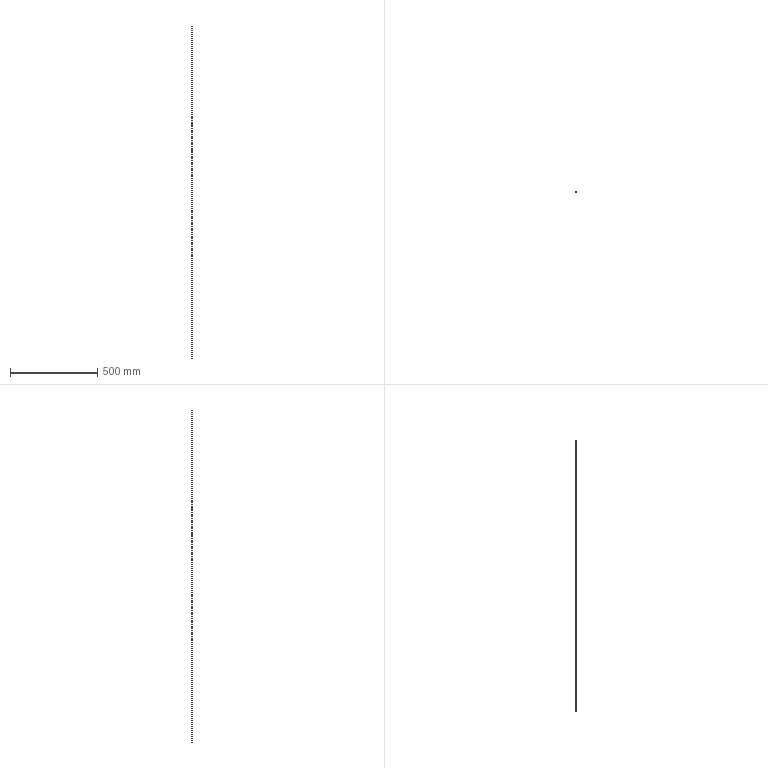Part | SolidWorks | features Extrusion 1 | 1 solid | 10 faces | box 3 x 3 x 1900 mm | volume 13027 mm3 | cylinder 8 | plane 2 | commonest cylinder face diameters 0.3 x6 3 x2
STEP:
#1=CARTESIAN_POINT('',(-0.9727,-0.475,1900.));
#2=VERTEX_POINT('',#1);
#3=CARTESIAN_POINT('',(-0.6727,-0.475,1900.));
#4=VERTEX_POINT('',#3);
#5=CARTESIAN_POINT('',(-0.8227,-0.475,1900.));
#6=DIRECTION('',(0.,0.,1.));
#7=DIRECTION('',(1.,0.,0.));
#8=AXIS2_PLACEMENT_3D('',#5,#6,#7);
#9=CIRCLE('',#8,0.15);
#10=EDGE_CURVE('',#2,#4,#9,.T.);
#11=ORIENTED_EDGE('',*,*,#10,.T.);
#12=CARTESIAN_POINT('',(-0.6727,-0.475,0.));
#13=VERTEX_POINT('',#12);
#14=CARTESIAN_POINT('',(-0.6727,-0.475,1900.));
#15=DIRECTION('',(0.,0.,-1.));
#16=VECTOR('',#15,1000.);
#17=LINE('',#14,#16);
#18=EDGE_CURVE('',#4,#13,#17,.T.);
#19=ORIENTED_EDGE('',*,*,#18,.T.);
#20=CARTESIAN_POINT('',(-0.9727,-0.475,0.));
#21=VERTEX_POINT('',#20);
#22=CARTESIAN_POINT('',(-0.8227,-0.475,0.));
#23=DIRECTION('',(0.,0.,1.));
#24=DIRECTION('',(1.,0.,0.));
#25=AXIS2_PLACEMENT_3D('',#22,#23,#24);
#26=CIRCLE('',#25,0.15);
#27=EDGE_CURVE('',#21,#13,#26,.T.);
#28=ORIENTED_EDGE('',*,*,#27,.F.);
#29=CARTESIAN_POINT('',(-0.9727,-0.475,1900.));
#30=DIRECTION('',(0.,0.,-1.));
#31=VECTOR('',#30,1000.);
#32=LINE('',#29,#31);
#33=EDGE_CURVE('',#2,#21,#32,.T.);
#34=ORIENTED_EDGE('',*,*,#33,.F.);
#35=EDGE_LOOP('',(#11,#19,#28,#34));
#36=FACE_OUTER_BOUND('',#35,.T.);
#37=CARTESIAN_POINT('',(-0.8227,-0.475,1900.));
#38=DIRECTION('',(0.,0.,-1.));
#39=DIRECTION('',(-1.,0.,0.));
#40=AXIS2_PLACEMENT_3D('',#37,#38,#39);
#41=CYLINDRICAL_SURFACE('',#40,0.15);
#42=ADVANCED_FACE('',(#36),#41,.F.);
#43=CARTESIAN_POINT('',(0.6727,-0.475,1900.));
#44=VERTEX_POINT('',#43);
#45=CARTESIAN_POINT('',(0.9727,-0.475,1900.));
#46=VERTEX_POINT('',#45);
#47=CARTESIAN_POINT('',(0.8227,-0.475,1900.));
#48=DIRECTION('',(0.,0.,1.));
#49=DIRECTION('',(1.,0.,0.));
#50=AXIS2_PLACEMENT_3D('',#47,#48,#49);
#51=CIRCLE('',#50,0.15);
#52=EDGE_CURVE('',#44,#46,#51,.T.);
#53=ORIENTED_EDGE('',*,*,#52,.T.);
#54=CARTESIAN_POINT('',(0.9727,-0.475,0.));
#55=VERTEX_POINT('',#54);
#56=CARTESIAN_POINT('',(0.9727,-0.475,1900.));
#57=DIRECTION('',(0.,0.,-1.));
#58=VECTOR('',#57,1000.);
#59=LINE('',#56,#58);
#60=EDGE_CURVE('',#46,#55,#59,.T.);
#61=ORIENTED_EDGE('',*,*,#60,.T.);
#62=CARTESIAN_POINT('',(0.6727,-0.475,0.));
#63=VERTEX_POINT('',#62);
#64=CARTESIAN_POINT('',(0.8227,-0.475,0.));
#65=DIRECTION('',(0.,0.,1.));
#66=DIRECTION('',(1.,0.,0.));
#67=AXIS2_PLACEMENT_3D('',#64,#65,#66);
#68=CIRCLE('',#67,0.15);
#69=EDGE_CURVE('',#63,#55,#68,.T.);
#70=ORIENTED_EDGE('',*,*,#69,.F.);
#71=CARTESIAN_POINT('',(0.6727,-0.475,1900.));
#72=DIRECTION('',(0.,0.,-1.));
#73=VECTOR('',#72,1000.);
#74=LINE('',#71,#73);
#75=EDGE_CURVE('',#44,#63,#74,.T.);
#76=ORIENTED_EDGE('',*,*,#75,.F.);
#77=EDGE_LOOP('',(#53,#61,#70,#76));
#78=FACE_OUTER_BOUND('',#77,.T.);
#79=CARTESIAN_POINT('',(0.8227,-0.475,1900.));
#80=DIRECTION('',(0.,0.,-1.));
#81=DIRECTION('',(-1.,0.,0.));
#82=AXIS2_PLACEMENT_3D('',#79,#80,#81);
#83=CYLINDRICAL_SURFACE('',#82,0.15);
#84=ADVANCED_FACE('',(#78),#83,.F.);
#85=CARTESIAN_POINT('',(-0.15,0.95,1900.));
#86=VERTEX_POINT('',#85);
#87=CARTESIAN_POINT('',(0.15,0.95,1900.));
#88=VERTEX_POINT('',#87);
#89=CARTESIAN_POINT('',(0.,0.95,1900.));
#90=DIRECTION('',(0.,0.,1.));
#91=DIRECTION('',(1.,0.,0.));
#92=AXIS2_PLACEMENT_3D('',#89,#90,#91);
#93=CIRCLE('',#92,0.15);
#94=EDGE_CURVE('',#86,#88,#93,.T.);
#95=ORIENTED_EDGE('',*,*,#94,.T.);
#96=CARTESIAN_POINT('',(0.15,0.95,0.));
#97=VERTEX_POINT('',#96);
#98=CARTESIAN_POINT('',(0.15,0.95,1900.));
#99=DIRECTION('',(0.,0.,-1.));
#100=VECTOR('',#99,1000.);
#101=LINE('',#98,#100);
#102=EDGE_CURVE('',#88,#97,#101,.T.);
#103=ORIENTED_EDGE('',*,*,#102,.T.);
#104=CARTESIAN_POINT('',(-0.15,0.95,0.));
#105=VERTEX_POINT('',#104);
#106=CARTESIAN_POINT('',(0.,0.95,0.));
#107=DIRECTION('',(0.,0.,1.));
#108=DIRECTION('',(1.,0.,0.));
#109=AXIS2_PLACEMENT_3D('',#106,#107,#108);
#110=CIRCLE('',#109,0.15);
#111=EDGE_CURVE('',#105,#97,#110,.T.);
#112=ORIENTED_EDGE('',*,*,#111,.F.);
#113=CARTESIAN_POINT('',(-0.15,0.95,1900.));
#114=DIRECTION('',(0.,0.,-1.));
#115=VECTOR('',#114,1000.);
#116=LINE('',#113,#115);
#117=EDGE_CURVE('',#86,#105,#116,.T.);
#118=ORIENTED_EDGE('',*,*,#117,.F.);
#119=EDGE_LOOP('',(#95,#103,#112,#118));
#120=FACE_OUTER_BOUND('',#119,.T.);
#121=CARTESIAN_POINT('',(0.,0.95,1900.));
#122=DIRECTION('',(0.,0.,-1.));
#123=DIRECTION('',(-1.,0.,0.));
#124=AXIS2_PLACEMENT_3D('',#121,#122,#123);
#125=CYLINDRICAL_SURFACE('',#124,0.15);
#126=ADVANCED_FACE('',(#120),#125,.F.);
#127=CARTESIAN_POINT('',(1.5,0.,1900.));
#128=VERTEX_POINT('',#127);
#129=CARTESIAN_POINT('',(-1.5,0.,1900.));
#130=VERTEX_POINT('',#129);
#131=CARTESIAN_POINT('',(0.,0.,1900.));
#132=DIRECTION('',(0.,0.,1.));
#133=DIRECTION('',(1.,0.,0.));
#134=AXIS2_PLACEMENT_3D('',#131,#132,#133);
#135=CIRCLE('',#134,1.5);
#136=EDGE_CURVE('',#128,#130,#135,.T.);
#137=ORIENTED_EDGE('',*,*,#136,.F.);
#138=CARTESIAN_POINT('',(1.5,0.,0.));
#139=VERTEX_POINT('',#138);
#140=CARTESIAN_POINT('',(1.5,0.,1900.));
#141=DIRECTION('',(0.,0.,-1.));
#142=VECTOR('',#141,1000.);
#143=LINE('',#140,#142);
#144=EDGE_CURVE('',#128,#139,#143,.T.);
#145=ORIENTED_EDGE('',*,*,#144,.T.);
#146=CARTESIAN_POINT('',(-1.5,0.,0.));
#147=VERTEX_POINT('',#146);
#148=CARTESIAN_POINT('',(0.,0.,0.));
#149=DIRECTION('',(0.,0.,1.));
#150=DIRECTION('',(1.,0.,0.));
#151=AXIS2_PLACEMENT_3D('',#148,#149,#150);
#152=CIRCLE('',#151,1.5);
#153=EDGE_CURVE('',#139,#147,#152,.T.);
#154=ORIENTED_EDGE('',*,*,#153,.T.);
#155=CARTESIAN_POINT('',(-1.5,0.,1900.));
#156=DIRECTION('',(0.,0.,-1.));
#157=VECTOR('',#156,1000.);
#158=LINE('',#155,#157);
#159=EDGE_CURVE('',#130,#147,#158,.T.);
#160=ORIENTED_EDGE('',*,*,#159,.F.);
#161=EDGE_LOOP('',(#137,#145,#154,#160));
#162=FACE_OUTER_BOUND('',#161,.T.);
#163=CARTESIAN_POINT('',(0.,0.,1900.));
#164=DIRECTION('',(0.,0.,-1.));
#165=DIRECTION('',(-1.,0.,0.));
#166=AXIS2_PLACEMENT_3D('',#163,#164,#165);
#167=CYLINDRICAL_SURFACE('',#166,1.5);
#168=ADVANCED_FACE('',(#162),#167,.T.);
#169=ORIENTED_EDGE('',*,*,#52,.F.);
#170=CARTESIAN_POINT('',(0.8227,-0.475,1900.));
#171=DIRECTION('',(0.,0.,1.));
#172=DIRECTION('',(1.,0.,0.));
#173=AXIS2_PLACEMENT_3D('',#170,#171,#172);
#174=CIRCLE('',#173,0.15);
#175=EDGE_CURVE('',#46,#44,#174,.T.);
#176=ORIENTED_EDGE('',*,*,#175,.F.);
#177=EDGE_LOOP('',(#169,#176));
#178=FACE_BOUND('',#177,.T.);
#179=CARTESIAN_POINT('',(0.,0.,1900.));
#180=DIRECTION('',(0.,0.,1.));
#181=DIRECTION('',(1.,0.,0.));
#182=AXIS2_PLACEMENT_3D('',#179,#180,#181);
#183=CIRCLE('',#182,1.5);
#184=EDGE_CURVE('',#130,#128,#183,.T.);
#185=ORIENTED_EDGE('',*,*,#184,.T.);
#186=ORIENTED_EDGE('',*,*,#136,.T.);
#187=EDGE_LOOP('',(#185,#186));
#188=FACE_OUTER_BOUND('',#187,.T.);
#189=ORIENTED_EDGE('',*,*,#94,.F.);
#190=CARTESIAN_POINT('',(0.,0.95,1900.));
#191=DIRECTION('',(0.,0.,1.));
#192=DIRECTION('',(1.,0.,0.));
#193=AXIS2_PLACEMENT_3D('',#190,#191,#192);
#194=CIRCLE('',#193,0.15);
#195=EDGE_CURVE('',#88,#86,#194,.T.);
#196=ORIENTED_EDGE('',*,*,#195,.F.);
#197=EDGE_LOOP('',(#189,#196));
#198=FACE_BOUND('',#197,.T.);
#199=ORIENTED_EDGE('',*,*,#10,.F.);
#200=CARTESIAN_POINT('',(-0.8227,-0.475,1900.));
#201=DIRECTION('',(0.,0.,1.));
#202=DIRECTION('',(1.,0.,0.));
#203=AXIS2_PLACEMENT_3D('',#200,#201,#202);
#204=CIRCLE('',#203,0.15);
#205=EDGE_CURVE('',#4,#2,#204,.T.);
#206=ORIENTED_EDGE('',*,*,#205,.F.);
#207=EDGE_LOOP('',(#199,#206));
#208=FACE_BOUND('',#207,.T.);
#209=CARTESIAN_POINT('',(0.,0.,1900.));
#210=DIRECTION('',(0.,0.,1.));
#211=DIRECTION('',(1.,0.,0.));
#212=AXIS2_PLACEMENT_3D('',#209,#210,#211);
#213=PLANE('',#212);
#214=ADVANCED_FACE('',(#178,#188,#198,#208),#213,.T.);
#215=CARTESIAN_POINT('',(0.,0.,0.));
#216=DIRECTION('',(0.,0.,1.));
#217=DIRECTION('',(1.,0.,0.));
#218=AXIS2_PLACEMENT_3D('',#215,#216,#217);
#219=CIRCLE('',#218,1.5);
#220=EDGE_CURVE('',#147,#139,#219,.T.);
#221=ORIENTED_EDGE('',*,*,#220,.F.);
#222=ORIENTED_EDGE('',*,*,#153,.F.);
#223=EDGE_LOOP('',(#221,#222));
#224=FACE_OUTER_BOUND('',#223,.T.);
#225=ORIENTED_EDGE('',*,*,#111,.T.);
#226=CARTESIAN_POINT('',(0.,0.95,0.));
#227=DIRECTION('',(0.,0.,1.));
#228=DIRECTION('',(1.,0.,0.));
#229=AXIS2_PLACEMENT_3D('',#226,#227,#228);
#230=CIRCLE('',#229,0.15);
#231=EDGE_CURVE('',#97,#105,#230,.T.);
#232=ORIENTED_EDGE('',*,*,#231,.T.);
#233=EDGE_LOOP('',(#225,#232));
#234=FACE_BOUND('',#233,.T.);
#235=ORIENTED_EDGE('',*,*,#69,.T.);
#236=CARTESIAN_POINT('',(0.8227,-0.475,0.));
#237=DIRECTION('',(0.,0.,1.));
#238=DIRECTION('',(1.,0.,0.));
#239=AXIS2_PLACEMENT_3D('',#236,#237,#238);
#240=CIRCLE('',#239,0.15);
#241=EDGE_CURVE('',#55,#63,#240,.T.);
#242=ORIENTED_EDGE('',*,*,#241,.T.);
#243=EDGE_LOOP('',(#235,#242));
#244=FACE_BOUND('',#243,.T.);
#245=ORIENTED_EDGE('',*,*,#27,.T.);
#246=CARTESIAN_POINT('',(-0.8227,-0.475,0.));
#247=DIRECTION('',(0.,0.,1.));
#248=DIRECTION('',(1.,0.,0.));
#249=AXIS2_PLACEMENT_3D('',#246,#247,#248);
#250=CIRCLE('',#249,0.15);
#251=EDGE_CURVE('',#13,#21,#250,.T.);
#252=ORIENTED_EDGE('',*,*,#251,.T.);
#253=EDGE_LOOP('',(#245,#252));
#254=FACE_BOUND('',#253,.T.);
#255=CARTESIAN_POINT('',(0.,0.,0.));
#256=DIRECTION('',(0.,0.,1.));
#257=DIRECTION('',(1.,0.,0.));
#258=AXIS2_PLACEMENT_3D('',#255,#256,#257);
#259=PLANE('',#258);
#260=ADVANCED_FACE('',(#224,#234,#244,#254),#259,.F.);
#261=ORIENTED_EDGE('',*,*,#144,.F.);
#262=ORIENTED_EDGE('',*,*,#184,.F.);
#263=ORIENTED_EDGE('',*,*,#159,.T.);
#264=ORIENTED_EDGE('',*,*,#220,.T.);
#265=EDGE_LOOP('',(#261,#262,#263,#264));
#266=FACE_OUTER_BOUND('',#265,.T.);
#267=CARTESIAN_POINT('',(0.,0.,1900.));
#268=DIRECTION('',(0.,0.,-1.));
#269=DIRECTION('',(-1.,0.,0.));
#270=AXIS2_PLACEMENT_3D('',#267,#268,#269);
#271=CYLINDRICAL_SURFACE('',#270,1.5);
#272=ADVANCED_FACE('',(#266),#271,.T.);
#273=ORIENTED_EDGE('',*,*,#102,.F.);
#274=ORIENTED_EDGE('',*,*,#195,.T.);
#275=ORIENTED_EDGE('',*,*,#117,.T.);
#276=ORIENTED_EDGE('',*,*,#231,.F.);
#277=EDGE_LOOP('',(#273,#274,#275,#276));
#278=FACE_OUTER_BOUND('',#277,.T.);
#279=CARTESIAN_POINT('',(0.,0.95,1900.));
#280=DIRECTION('',(0.,0.,-1.));
#281=DIRECTION('',(-1.,0.,0.));
#282=AXIS2_PLACEMENT_3D('',#279,#280,#281);
#283=CYLINDRICAL_SURFACE('',#282,0.15);
#284=ADVANCED_FACE('',(#278),#283,.F.);
#285=ORIENTED_EDGE('',*,*,#60,.F.);
#286=ORIENTED_EDGE('',*,*,#175,.T.);
#287=ORIENTED_EDGE('',*,*,#75,.T.);
#288=ORIENTED_EDGE('',*,*,#241,.F.);
#289=EDGE_LOOP('',(#285,#286,#287,#288));
#290=FACE_OUTER_BOUND('',#289,.T.);
#291=CARTESIAN_POINT('',(0.8227,-0.475,1900.));
#292=DIRECTION('',(0.,0.,-1.));
#293=DIRECTION('',(-1.,0.,0.));
#294=AXIS2_PLACEMENT_3D('',#291,#292,#293);
#295=CYLINDRICAL_SURFACE('',#294,0.15);
#296=ADVANCED_FACE('',(#290),#295,.F.);
#297=ORIENTED_EDGE('',*,*,#18,.F.);
#298=ORIENTED_EDGE('',*,*,#205,.T.);
#299=ORIENTED_EDGE('',*,*,#33,.T.);
#300=ORIENTED_EDGE('',*,*,#251,.F.);
#301=EDGE_LOOP('',(#297,#298,#299,#300));
#302=FACE_OUTER_BOUND('',#301,.T.);
#303=CARTESIAN_POINT('',(-0.8227,-0.475,1900.));
#304=DIRECTION('',(0.,0.,-1.));
#305=DIRECTION('',(-1.,0.,0.));
#306=AXIS2_PLACEMENT_3D('',#303,#304,#305);
#307=CYLINDRICAL_SURFACE('',#306,0.15);
#308=ADVANCED_FACE('',(#302),#307,.F.);
#309=CLOSED_SHELL('',(#42,#84,#126,#168,#214,#260,#272,#284,#296,#308));
#310=MANIFOLD_SOLID_BREP('',#309);
#311=CARTESIAN_POINT('',(0.,0.,0.));
#312=DIRECTION('',(0.,0.,1.));
#313=DIRECTION('',(1.,0.,0.));
#314=AXIS2_PLACEMENT_3D('',#311,#312,#313);
#315=(LENGTH_UNIT()NAMED_UNIT(*)SI_UNIT(.MILLI.,.METRE.));
#316=UNCERTAINTY_MEASURE_WITH_UNIT(LENGTH_MEASURE(0.00001),#315,'','');
#317=(NAMED_UNIT(*)PLANE_ANGLE_UNIT()SI_UNIT($,.RADIAN.));
#318=(NAMED_UNIT(*)SI_UNIT($,.STERADIAN.)SOLID_ANGLE_UNIT());
#319=(GEOMETRIC_REPRESENTATION_CONTEXT(3)GLOBAL_UNCERTAINTY_ASSIGNED_CONTEXT((#316))GLOBAL_UNIT_ASSIGNED_CONTEXT((#315,#317,#318))REPRESENTATION_CONTEXT('',''));
#320=ADVANCED_BREP_SHAPE_REPRESENTATION('',(#310,#314),#319);